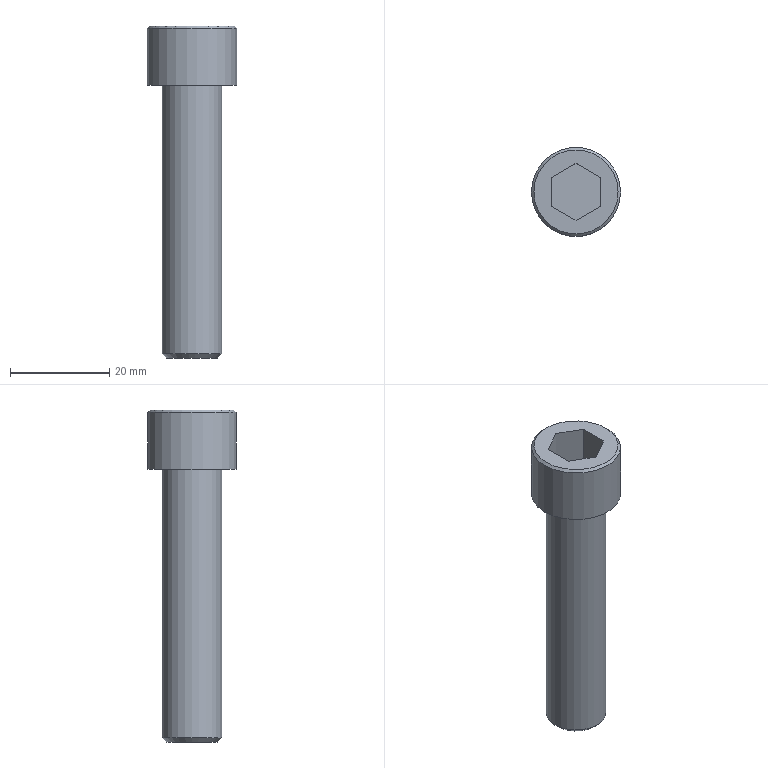Part | STEP file | gslz 2016.10.28-6_id90_x_t | 1 solid | 14 faces | box 18 x 18 x 67 mm | volume 8561 mm3 | plane 10 | cylinder 2 | cone 2 | commonest cylinder face diameters 12 x1 18 x1
STEP:
#1=CARTESIAN_POINT('',(-236.5,20.,-3.));
#2=VERTEX_POINT('',#1);
#3=CARTESIAN_POINT('',(-245.,20.,-3.));
#4=DIRECTION('',(0.,0.,1.));
#5=DIRECTION('',(1.,0.,0.));
#6=AXIS2_PLACEMENT_3D('',#3,#4,#5);
#7=CIRCLE('',#6,8.5);
#8=EDGE_CURVE('',#2,#2,#7,.T.);
#9=ORIENTED_EDGE('',*,*,#8,.T.);
#10=EDGE_LOOP('',(#9));
#11=FACE_BOUND('',#10,.T.);
#12=CARTESIAN_POINT('',(-250.,22.887,-3.));
#13=VERTEX_POINT('',#12);
#14=CARTESIAN_POINT('',(-250.,17.113,-3.));
#15=VERTEX_POINT('',#14);
#16=CARTESIAN_POINT('',(-250.,22.887,-3.));
#17=DIRECTION('',(0.,-1.,0.));
#18=VECTOR('',#17,1.);
#19=LINE('',#16,#18);
#20=EDGE_CURVE('',#13,#15,#19,.T.);
#21=ORIENTED_EDGE('',*,*,#20,.F.);
#22=CARTESIAN_POINT('',(-245.,25.774,-3.));
#23=VERTEX_POINT('',#22);
#24=CARTESIAN_POINT('',(-245.,25.774,-3.));
#25=DIRECTION('',(-0.866,-0.5,0.));
#26=VECTOR('',#25,1.);
#27=LINE('',#24,#26);
#28=EDGE_CURVE('',#23,#13,#27,.T.);
#29=ORIENTED_EDGE('',*,*,#28,.F.);
#30=CARTESIAN_POINT('',(-240.,22.887,-3.));
#31=VERTEX_POINT('',#30);
#32=CARTESIAN_POINT('',(-240.,22.887,-3.));
#33=DIRECTION('',(-0.866,0.5,0.));
#34=VECTOR('',#33,1.);
#35=LINE('',#32,#34);
#36=EDGE_CURVE('',#31,#23,#35,.T.);
#37=ORIENTED_EDGE('',*,*,#36,.F.);
#38=CARTESIAN_POINT('',(-240.,17.113,-3.));
#39=VERTEX_POINT('',#38);
#40=CARTESIAN_POINT('',(-240.,17.113,-3.));
#41=DIRECTION('',(0.,1.,0.));
#42=VECTOR('',#41,1.);
#43=LINE('',#40,#42);
#44=EDGE_CURVE('',#39,#31,#43,.T.);
#45=ORIENTED_EDGE('',*,*,#44,.F.);
#46=CARTESIAN_POINT('',(-245.,14.226,-3.));
#47=VERTEX_POINT('',#46);
#48=CARTESIAN_POINT('',(-245.,14.226,-3.));
#49=DIRECTION('',(0.866,0.5,0.));
#50=VECTOR('',#49,1.);
#51=LINE('',#48,#50);
#52=EDGE_CURVE('',#47,#39,#51,.T.);
#53=ORIENTED_EDGE('',*,*,#52,.F.);
#54=CARTESIAN_POINT('',(-250.,17.113,-3.));
#55=DIRECTION('',(0.866,-0.5,0.));
#56=VECTOR('',#55,1.);
#57=LINE('',#54,#56);
#58=EDGE_CURVE('',#15,#47,#57,.T.);
#59=ORIENTED_EDGE('',*,*,#58,.F.);
#60=EDGE_LOOP('',(#21,#29,#37,#45,#53,#59));
#61=FACE_BOUND('',#60,.T.);
#62=CARTESIAN_POINT('',(-245.,20.,-3.));
#63=DIRECTION('',(0.,0.,1.));
#64=DIRECTION('',(-1.,0.,0.));
#65=AXIS2_PLACEMENT_3D('',#62,#63,#64);
#66=PLANE('',#65);
#67=ADVANCED_FACE('',(#11,#61),#66,.T.);
#68=CARTESIAN_POINT('',(-250.15,20.,-70.));
#69=VERTEX_POINT('',#68);
#70=CARTESIAN_POINT('',(-245.,20.,-70.));
#71=DIRECTION('',(0.,0.,-1.));
#72=DIRECTION('',(-1.,0.,0.));
#73=AXIS2_PLACEMENT_3D('',#70,#71,#72);
#74=CIRCLE('',#73,5.15);
#75=EDGE_CURVE('',#69,#69,#74,.T.);
#76=ORIENTED_EDGE('',*,*,#75,.T.);
#77=EDGE_LOOP('',(#76));
#78=FACE_OUTER_BOUND('',#77,.T.);
#79=CARTESIAN_POINT('',(-245.,20.,-70.));
#80=DIRECTION('',(0.,0.,-1.));
#81=DIRECTION('',(1.,0.,0.));
#82=AXIS2_PLACEMENT_3D('',#79,#80,#81);
#83=PLANE('',#82);
#84=ADVANCED_FACE('',(#78),#83,.T.);
#85=CARTESIAN_POINT('',(-251.,20.,-69.15));
#86=VERTEX_POINT('',#85);
#87=CARTESIAN_POINT('',(-245.,20.,-69.15));
#88=DIRECTION('',(0.,0.,1.));
#89=DIRECTION('',(-1.,0.,0.));
#90=AXIS2_PLACEMENT_3D('',#87,#88,#89);
#91=CIRCLE('',#90,6.);
#92=EDGE_CURVE('',#86,#86,#91,.T.);
#93=ORIENTED_EDGE('',*,*,#92,.T.);
#94=EDGE_LOOP('',(#93));
#95=FACE_BOUND('',#94,.T.);
#96=CARTESIAN_POINT('',(-251.,20.,-15.));
#97=VERTEX_POINT('',#96);
#98=CARTESIAN_POINT('',(-245.,20.,-15.));
#99=DIRECTION('',(0.,0.,-1.));
#100=DIRECTION('',(-1.,0.,0.));
#101=AXIS2_PLACEMENT_3D('',#98,#99,#100);
#102=CIRCLE('',#101,6.);
#103=EDGE_CURVE('',#97,#97,#102,.T.);
#104=ORIENTED_EDGE('',*,*,#103,.T.);
#105=EDGE_LOOP('',(#104));
#106=FACE_BOUND('',#105,.T.);
#107=CARTESIAN_POINT('',(-245.,20.,-50.));
#108=DIRECTION('',(0.,0.,-1.));
#109=DIRECTION('',(-1.,0.,0.));
#110=AXIS2_PLACEMENT_3D('',#107,#108,#109);
#111=CYLINDRICAL_SURFACE('',#110,6.);
#112=ADVANCED_FACE('',(#95,#106),#111,.T.);
#113=ORIENTED_EDGE('',*,*,#103,.F.);
#114=EDGE_LOOP('',(#113));
#115=FACE_BOUND('',#114,.T.);
#116=CARTESIAN_POINT('',(-254.,20.,-15.));
#117=VERTEX_POINT('',#116);
#118=CARTESIAN_POINT('',(-245.,20.,-15.));
#119=DIRECTION('',(0.,0.,-1.));
#120=DIRECTION('',(-1.,0.,0.));
#121=AXIS2_PLACEMENT_3D('',#118,#119,#120);
#122=CIRCLE('',#121,9.);
#123=EDGE_CURVE('',#117,#117,#122,.T.);
#124=ORIENTED_EDGE('',*,*,#123,.T.);
#125=EDGE_LOOP('',(#124));
#126=FACE_BOUND('',#125,.T.);
#127=CARTESIAN_POINT('',(-245.,20.,-15.));
#128=DIRECTION('',(0.,0.,-1.));
#129=DIRECTION('',(1.,0.,0.));
#130=AXIS2_PLACEMENT_3D('',#127,#128,#129);
#131=PLANE('',#130);
#132=ADVANCED_FACE('',(#115,#126),#131,.T.);
#133=CARTESIAN_POINT('',(-236.,20.,-3.5));
#134=VERTEX_POINT('',#133);
#135=CARTESIAN_POINT('',(-245.,20.,-3.5));
#136=DIRECTION('',(0.,0.,-1.));
#137=DIRECTION('',(1.,0.,0.));
#138=AXIS2_PLACEMENT_3D('',#135,#136,#137);
#139=CIRCLE('',#138,9.);
#140=EDGE_CURVE('',#134,#134,#139,.T.);
#141=ORIENTED_EDGE('',*,*,#140,.T.);
#142=EDGE_LOOP('',(#141));
#143=FACE_BOUND('',#142,.T.);
#144=ORIENTED_EDGE('',*,*,#123,.F.);
#145=EDGE_LOOP('',(#144));
#146=FACE_BOUND('',#145,.T.);
#147=CARTESIAN_POINT('',(-245.,20.,0.));
#148=DIRECTION('',(0.,0.,-1.));
#149=DIRECTION('',(-1.,0.,0.));
#150=AXIS2_PLACEMENT_3D('',#147,#148,#149);
#151=CYLINDRICAL_SURFACE('',#150,9.);
#152=ADVANCED_FACE('',(#143,#146),#151,.T.);
#153=ORIENTED_EDGE('',*,*,#92,.F.);
#154=EDGE_LOOP('',(#153));
#155=FACE_BOUND('',#154,.T.);
#156=ORIENTED_EDGE('',*,*,#75,.F.);
#157=EDGE_LOOP('',(#156));
#158=FACE_BOUND('',#157,.T.);
#159=CARTESIAN_POINT('',(-245.,20.,-70.));
#160=DIRECTION('',(0.,0.,1.));
#161=DIRECTION('',(1.,0.,0.));
#162=AXIS2_PLACEMENT_3D('',#159,#160,#161);
#163=CONICAL_SURFACE('',#162,5.15,45.);
#164=ADVANCED_FACE('',(#155,#158),#163,.T.);
#165=ORIENTED_EDGE('',*,*,#20,.T.);
#166=CARTESIAN_POINT('',(-250.,17.113,-11.));
#167=VERTEX_POINT('',#166);
#168=CARTESIAN_POINT('',(-250.,17.113,-11.));
#169=DIRECTION('',(0.,0.,-1.));
#170=VECTOR('',#169,1.);
#171=LINE('',#168,#170);
#172=EDGE_CURVE('',#15,#167,#171,.T.);
#173=ORIENTED_EDGE('',*,*,#172,.T.);
#174=CARTESIAN_POINT('',(-250.,22.887,-11.));
#175=VERTEX_POINT('',#174);
#176=CARTESIAN_POINT('',(-250.,22.887,-11.));
#177=DIRECTION('',(0.,1.,0.));
#178=VECTOR('',#177,1.);
#179=LINE('',#176,#178);
#180=EDGE_CURVE('',#167,#175,#179,.T.);
#181=ORIENTED_EDGE('',*,*,#180,.T.);
#182=CARTESIAN_POINT('',(-250.,22.887,-11.));
#183=DIRECTION('',(0.,0.,-1.));
#184=VECTOR('',#183,1.);
#185=LINE('',#182,#184);
#186=EDGE_CURVE('',#13,#175,#185,.T.);
#187=ORIENTED_EDGE('',*,*,#186,.F.);
#188=EDGE_LOOP('',(#165,#173,#181,#187));
#189=FACE_OUTER_BOUND('',#188,.T.);
#190=CARTESIAN_POINT('',(-250.,22.887,-11.));
#191=DIRECTION('',(-1.,0.,0.));
#192=DIRECTION('',(0.,0.,1.));
#193=AXIS2_PLACEMENT_3D('',#190,#191,#192);
#194=PLANE('',#193);
#195=ADVANCED_FACE('',(#189),#194,.F.);
#196=ORIENTED_EDGE('',*,*,#58,.T.);
#197=CARTESIAN_POINT('',(-245.,14.226,-11.));
#198=VERTEX_POINT('',#197);
#199=CARTESIAN_POINT('',(-245.,14.226,-11.));
#200=DIRECTION('',(0.,0.,-1.));
#201=VECTOR('',#200,1.);
#202=LINE('',#199,#201);
#203=EDGE_CURVE('',#47,#198,#202,.T.);
#204=ORIENTED_EDGE('',*,*,#203,.T.);
#205=CARTESIAN_POINT('',(-250.,17.113,-11.));
#206=DIRECTION('',(-0.866,0.5,0.));
#207=VECTOR('',#206,1.);
#208=LINE('',#205,#207);
#209=EDGE_CURVE('',#198,#167,#208,.T.);
#210=ORIENTED_EDGE('',*,*,#209,.T.);
#211=ORIENTED_EDGE('',*,*,#172,.F.);
#212=EDGE_LOOP('',(#196,#204,#210,#211));
#213=FACE_OUTER_BOUND('',#212,.T.);
#214=CARTESIAN_POINT('',(-250.,17.113,-11.));
#215=DIRECTION('',(-0.5,-0.866,0.));
#216=DIRECTION('',(-0.866,0.5,0.));
#217=AXIS2_PLACEMENT_3D('',#214,#215,#216);
#218=PLANE('',#217);
#219=ADVANCED_FACE('',(#213),#218,.F.);
#220=ORIENTED_EDGE('',*,*,#52,.T.);
#221=CARTESIAN_POINT('',(-240.,17.113,-11.));
#222=VERTEX_POINT('',#221);
#223=CARTESIAN_POINT('',(-240.,17.113,-11.));
#224=DIRECTION('',(0.,0.,-1.));
#225=VECTOR('',#224,1.);
#226=LINE('',#223,#225);
#227=EDGE_CURVE('',#39,#222,#226,.T.);
#228=ORIENTED_EDGE('',*,*,#227,.T.);
#229=CARTESIAN_POINT('',(-245.,14.226,-11.));
#230=DIRECTION('',(-0.866,-0.5,0.));
#231=VECTOR('',#230,1.);
#232=LINE('',#229,#231);
#233=EDGE_CURVE('',#222,#198,#232,.T.);
#234=ORIENTED_EDGE('',*,*,#233,.T.);
#235=ORIENTED_EDGE('',*,*,#203,.F.);
#236=EDGE_LOOP('',(#220,#228,#234,#235));
#237=FACE_OUTER_BOUND('',#236,.T.);
#238=CARTESIAN_POINT('',(-245.,14.226,-11.));
#239=DIRECTION('',(0.5,-0.866,0.));
#240=DIRECTION('',(-0.866,-0.5,0.));
#241=AXIS2_PLACEMENT_3D('',#238,#239,#240);
#242=PLANE('',#241);
#243=ADVANCED_FACE('',(#237),#242,.F.);
#244=ORIENTED_EDGE('',*,*,#44,.T.);
#245=CARTESIAN_POINT('',(-240.,22.887,-11.));
#246=VERTEX_POINT('',#245);
#247=CARTESIAN_POINT('',(-240.,22.887,-11.));
#248=DIRECTION('',(0.,0.,-1.));
#249=VECTOR('',#248,1.);
#250=LINE('',#247,#249);
#251=EDGE_CURVE('',#31,#246,#250,.T.);
#252=ORIENTED_EDGE('',*,*,#251,.T.);
#253=CARTESIAN_POINT('',(-240.,17.113,-11.));
#254=DIRECTION('',(0.,-1.,0.));
#255=VECTOR('',#254,1.);
#256=LINE('',#253,#255);
#257=EDGE_CURVE('',#246,#222,#256,.T.);
#258=ORIENTED_EDGE('',*,*,#257,.T.);
#259=ORIENTED_EDGE('',*,*,#227,.F.);
#260=EDGE_LOOP('',(#244,#252,#258,#259));
#261=FACE_OUTER_BOUND('',#260,.T.);
#262=CARTESIAN_POINT('',(-240.,17.113,-11.));
#263=DIRECTION('',(1.,0.,0.));
#264=DIRECTION('',(0.,0.,1.));
#265=AXIS2_PLACEMENT_3D('',#262,#263,#264);
#266=PLANE('',#265);
#267=ADVANCED_FACE('',(#261),#266,.F.);
#268=ORIENTED_EDGE('',*,*,#36,.T.);
#269=CARTESIAN_POINT('',(-245.,25.774,-11.));
#270=VERTEX_POINT('',#269);
#271=CARTESIAN_POINT('',(-245.,25.774,-11.));
#272=DIRECTION('',(0.,0.,-1.));
#273=VECTOR('',#272,1.);
#274=LINE('',#271,#273);
#275=EDGE_CURVE('',#23,#270,#274,.T.);
#276=ORIENTED_EDGE('',*,*,#275,.T.);
#277=CARTESIAN_POINT('',(-240.,22.887,-11.));
#278=DIRECTION('',(0.866,-0.5,0.));
#279=VECTOR('',#278,1.);
#280=LINE('',#277,#279);
#281=EDGE_CURVE('',#270,#246,#280,.T.);
#282=ORIENTED_EDGE('',*,*,#281,.T.);
#283=ORIENTED_EDGE('',*,*,#251,.F.);
#284=EDGE_LOOP('',(#268,#276,#282,#283));
#285=FACE_OUTER_BOUND('',#284,.T.);
#286=CARTESIAN_POINT('',(-240.,22.887,-11.));
#287=DIRECTION('',(0.5,0.866,0.));
#288=DIRECTION('',(0.866,-0.5,0.));
#289=AXIS2_PLACEMENT_3D('',#286,#287,#288);
#290=PLANE('',#289);
#291=ADVANCED_FACE('',(#285),#290,.F.);
#292=ORIENTED_EDGE('',*,*,#28,.T.);
#293=ORIENTED_EDGE('',*,*,#186,.T.);
#294=CARTESIAN_POINT('',(-245.,25.774,-11.));
#295=DIRECTION('',(0.866,0.5,0.));
#296=VECTOR('',#295,1.);
#297=LINE('',#294,#296);
#298=EDGE_CURVE('',#175,#270,#297,.T.);
#299=ORIENTED_EDGE('',*,*,#298,.T.);
#300=ORIENTED_EDGE('',*,*,#275,.F.);
#301=EDGE_LOOP('',(#292,#293,#299,#300));
#302=FACE_OUTER_BOUND('',#301,.T.);
#303=CARTESIAN_POINT('',(-245.,25.774,-11.));
#304=DIRECTION('',(-0.5,0.866,0.));
#305=DIRECTION('',(0.866,0.5,0.));
#306=AXIS2_PLACEMENT_3D('',#303,#304,#305);
#307=PLANE('',#306);
#308=ADVANCED_FACE('',(#302),#307,.F.);
#309=ORIENTED_EDGE('',*,*,#180,.F.);
#310=ORIENTED_EDGE('',*,*,#209,.F.);
#311=ORIENTED_EDGE('',*,*,#233,.F.);
#312=ORIENTED_EDGE('',*,*,#257,.F.);
#313=ORIENTED_EDGE('',*,*,#281,.F.);
#314=ORIENTED_EDGE('',*,*,#298,.F.);
#315=EDGE_LOOP('',(#309,#310,#311,#312,#313,#314));
#316=FACE_OUTER_BOUND('',#315,.T.);
#317=CARTESIAN_POINT('',(-250.,17.113,-11.));
#318=DIRECTION('',(0.,0.,1.));
#319=DIRECTION('',(-1.,0.,0.));
#320=AXIS2_PLACEMENT_3D('',#317,#318,#319);
#321=PLANE('',#320);
#322=ADVANCED_FACE('',(#316),#321,.T.);
#323=ORIENTED_EDGE('',*,*,#8,.F.);
#324=EDGE_LOOP('',(#323));
#325=FACE_BOUND('',#324,.T.);
#326=ORIENTED_EDGE('',*,*,#140,.F.);
#327=EDGE_LOOP('',(#326));
#328=FACE_BOUND('',#327,.T.);
#329=CARTESIAN_POINT('',(-245.,20.,-3.5));
#330=DIRECTION('',(0.,0.,-1.));
#331=DIRECTION('',(-1.,0.,0.));
#332=AXIS2_PLACEMENT_3D('',#329,#330,#331);
#333=CONICAL_SURFACE('',#332,9.,45.);
#334=ADVANCED_FACE('',(#325,#328),#333,.T.);
#335=CLOSED_SHELL('',(#67,#84,#112,#132,#152,#164,#195,#219,#243,#267,#291,#308,#322,#334));
#336=MANIFOLD_SOLID_BREP('',#335);
#337=(LENGTH_UNIT()NAMED_UNIT(*)SI_UNIT(.MILLI.,.METRE.));
#338=UNCERTAINTY_MEASURE_WITH_UNIT(LENGTH_MEASURE(0.00002),#337,'','');
#339=(NAMED_UNIT(*)PLANE_ANGLE_UNIT()SI_UNIT($,.RADIAN.));
#340=PLANE_ANGLE_MEASURE_WITH_UNIT(PLANE_ANGLE_MEASURE(0.01745),#339);
#341=DIMENSIONAL_EXPONENTS(0.,0.,0.,0.,0.,0.,0.);
#342=(CONVERSION_BASED_UNIT('DEGREE',#340)NAMED_UNIT(#341)PLANE_ANGLE_UNIT());
#343=(NAMED_UNIT(*)SI_UNIT($,.STERADIAN.)SOLID_ANGLE_UNIT());
#344=(GEOMETRIC_REPRESENTATION_CONTEXT(3)GLOBAL_UNCERTAINTY_ASSIGNED_CONTEXT((#338))GLOBAL_UNIT_ASSIGNED_CONTEXT((#337,#342,#343))REPRESENTATION_CONTEXT('',''));
#345=ADVANCED_BREP_SHAPE_REPRESENTATION('',(#336),#344);